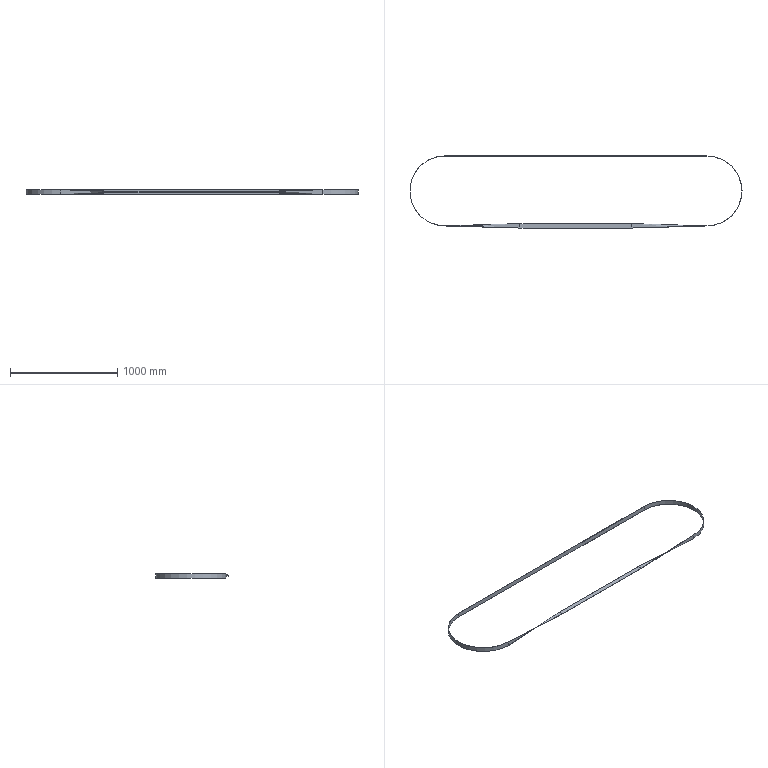Part | SolidWorks | features Blend 2, ICE 1, Sweep 1 | 1 solid | 26 faces | box 3091 x 670.5 x 43 mm | volume 356938 mm3 | plane 12 | spline 8 | cylinder 6 | commonest cylinder face diameters 648.7 x3 651.3 x3
STEP:
#1=CARTESIAN_POINT('',(0.,-325.65,-21.5));
#2=VERTEX_POINT('',#1);
#3=CARTESIAN_POINT('',(325.65,0.,-21.5));
#4=VERTEX_POINT('',#3);
#5=CARTESIAN_POINT('',(0.,0.,-21.5));
#6=DIRECTION('',(0.,0.,1.));
#7=DIRECTION('',(0.,-1.,0.));
#8=AXIS2_PLACEMENT_3D('',#5,#6,#7);
#9=CIRCLE('',#8,325.65);
#10=EDGE_CURVE('',#2,#4,#9,.T.);
#11=ORIENTED_EDGE('',*,*,#10,.T.);
#12=CARTESIAN_POINT('',(325.65,0.,21.5));
#13=VERTEX_POINT('',#12);
#14=CARTESIAN_POINT('',(325.65,0.,0.));
#15=DIRECTION('',(0.,0.,1.));
#16=VECTOR('',#15,1000.);
#17=LINE('',#14,#16);
#18=EDGE_CURVE('',#4,#13,#17,.T.);
#19=ORIENTED_EDGE('',*,*,#18,.T.);
#20=CARTESIAN_POINT('',(0.,-325.65,21.5));
#21=VERTEX_POINT('',#20);
#22=CARTESIAN_POINT('',(0.,0.,21.5));
#23=DIRECTION('',(0.,0.,1.));
#24=DIRECTION('',(0.,-1.,0.));
#25=AXIS2_PLACEMENT_3D('',#22,#23,#24);
#26=CIRCLE('',#25,325.65);
#27=EDGE_CURVE('',#21,#13,#26,.T.);
#28=ORIENTED_EDGE('',*,*,#27,.F.);
#29=CARTESIAN_POINT('',(0.,-325.65,1.363));
#30=VERTEX_POINT('',#29);
#31=CARTESIAN_POINT('',(0.,-325.65,-21.5));
#32=DIRECTION('',(0.,0.,1.));
#33=VECTOR('',#32,1000.);
#34=LINE('',#31,#33);
#35=EDGE_CURVE('',#30,#21,#34,.T.);
#36=ORIENTED_EDGE('',*,*,#35,.F.);
#37=CARTESIAN_POINT('',(0.,-325.65,-21.5));
#38=DIRECTION('',(0.,0.,1.));
#39=VECTOR('',#38,1000.);
#40=LINE('',#37,#39);
#41=EDGE_CURVE('',#2,#30,#40,.T.);
#42=ORIENTED_EDGE('',*,*,#41,.F.);
#43=EDGE_LOOP('',(#11,#19,#28,#36,#42));
#44=FACE_OUTER_BOUND('',#43,.T.);
#45=CARTESIAN_POINT('',(0.,0.,0.));
#46=DIRECTION('',(0.,0.,1.));
#47=DIRECTION('',(1.,0.,0.));
#48=AXIS2_PLACEMENT_3D('',#45,#46,#47);
#49=CYLINDRICAL_SURFACE('',#48,325.65);
#50=ADVANCED_FACE('',(#44),#49,.T.);
#51=CARTESIAN_POINT('',(324.35,0.,-21.5));
#52=VERTEX_POINT('',#51);
#53=CARTESIAN_POINT('',(0.,324.35,-21.5));
#54=VERTEX_POINT('',#53);
#55=CARTESIAN_POINT('',(0.,0.,-21.5));
#56=DIRECTION('',(0.,0.,1.));
#57=DIRECTION('',(0.,-1.,0.));
#58=AXIS2_PLACEMENT_3D('',#55,#56,#57);
#59=CIRCLE('',#58,324.35);
#60=EDGE_CURVE('',#52,#54,#59,.T.);
#61=ORIENTED_EDGE('',*,*,#60,.F.);
#62=CARTESIAN_POINT('',(324.35,0.,21.5));
#63=VERTEX_POINT('',#62);
#64=CARTESIAN_POINT('',(324.35,0.,0.));
#65=DIRECTION('',(0.,0.,1.));
#66=VECTOR('',#65,1000.);
#67=LINE('',#64,#66);
#68=EDGE_CURVE('',#52,#63,#67,.T.);
#69=ORIENTED_EDGE('',*,*,#68,.T.);
#70=CARTESIAN_POINT('',(0.,324.35,21.5));
#71=VERTEX_POINT('',#70);
#72=CARTESIAN_POINT('',(0.,0.,21.5));
#73=DIRECTION('',(0.,0.,1.));
#74=DIRECTION('',(0.,-1.,0.));
#75=AXIS2_PLACEMENT_3D('',#72,#73,#74);
#76=CIRCLE('',#75,324.35);
#77=EDGE_CURVE('',#63,#71,#76,.T.);
#78=ORIENTED_EDGE('',*,*,#77,.T.);
#79=CARTESIAN_POINT('',(0.,324.35,-21.5));
#80=DIRECTION('',(0.,0.,-1.));
#81=VECTOR('',#80,1000.);
#82=LINE('',#79,#81);
#83=EDGE_CURVE('',#71,#54,#82,.T.);
#84=ORIENTED_EDGE('',*,*,#83,.T.);
#85=EDGE_LOOP('',(#61,#69,#78,#84));
#86=FACE_OUTER_BOUND('',#85,.T.);
#87=CARTESIAN_POINT('',(0.,0.,0.));
#88=DIRECTION('',(0.,0.,1.));
#89=DIRECTION('',(1.,0.,0.));
#90=AXIS2_PLACEMENT_3D('',#87,#88,#89);
#91=CYLINDRICAL_SURFACE('',#90,324.35);
#92=ADVANCED_FACE('',(#86),#91,.F.);
#93=CARTESIAN_POINT('',(-2440.,-325.65,-21.5));
#94=VERTEX_POINT('',#93);
#95=CARTESIAN_POINT('',(-2440.,-325.65,21.5));
#96=VERTEX_POINT('',#95);
#97=CARTESIAN_POINT('',(-2440.,-325.65,-21.5));
#98=DIRECTION('',(0.,0.,1.));
#99=VECTOR('',#98,1000.);
#100=LINE('',#97,#99);
#101=EDGE_CURVE('',#94,#96,#100,.T.);
#102=ORIENTED_EDGE('',*,*,#101,.T.);
#103=CARTESIAN_POINT('',(-2440.,325.65,21.5));
#104=VERTEX_POINT('',#103);
#105=CARTESIAN_POINT('',(-2440.,0.,21.5));
#106=DIRECTION('',(0.,0.,1.));
#107=DIRECTION('',(0.,1.,0.));
#108=AXIS2_PLACEMENT_3D('',#105,#106,#107);
#109=CIRCLE('',#108,325.65);
#110=EDGE_CURVE('',#104,#96,#109,.T.);
#111=ORIENTED_EDGE('',*,*,#110,.F.);
#112=CARTESIAN_POINT('',(-2440.,325.65,-21.5));
#113=VERTEX_POINT('',#112);
#114=CARTESIAN_POINT('',(-2440.,325.65,-21.5));
#115=DIRECTION('',(0.,0.,1.));
#116=VECTOR('',#115,1000.);
#117=LINE('',#114,#116);
#118=EDGE_CURVE('',#113,#104,#117,.T.);
#119=ORIENTED_EDGE('',*,*,#118,.F.);
#120=CARTESIAN_POINT('',(-2440.,0.,-21.5));
#121=DIRECTION('',(0.,0.,1.));
#122=DIRECTION('',(0.,1.,0.));
#123=AXIS2_PLACEMENT_3D('',#120,#121,#122);
#124=CIRCLE('',#123,325.65);
#125=EDGE_CURVE('',#113,#94,#124,.T.);
#126=ORIENTED_EDGE('',*,*,#125,.T.);
#127=EDGE_LOOP('',(#102,#111,#119,#126));
#128=FACE_OUTER_BOUND('',#127,.T.);
#129=CARTESIAN_POINT('',(-2440.,0.,0.));
#130=DIRECTION('',(0.,0.,1.));
#131=DIRECTION('',(1.,0.,0.));
#132=AXIS2_PLACEMENT_3D('',#129,#130,#131);
#133=CYLINDRICAL_SURFACE('',#132,325.65);
#134=ADVANCED_FACE('',(#128),#133,.T.);
#135=ORIENTED_EDGE('',*,*,#125,.F.);
#136=CARTESIAN_POINT('',(-2440.,324.35,-21.5));
#137=VERTEX_POINT('',#136);
#138=CARTESIAN_POINT('',(-2440.,325.65,-21.5));
#139=DIRECTION('',(0.,1.,0.));
#140=VECTOR('',#139,1000.);
#141=LINE('',#138,#140);
#142=EDGE_CURVE('',#137,#113,#141,.T.);
#143=ORIENTED_EDGE('',*,*,#142,.F.);
#144=CARTESIAN_POINT('',(-2440.,-324.35,-21.5));
#145=VERTEX_POINT('',#144);
#146=CARTESIAN_POINT('',(-2440.,0.,-21.5));
#147=DIRECTION('',(0.,0.,1.));
#148=DIRECTION('',(0.,1.,0.));
#149=AXIS2_PLACEMENT_3D('',#146,#147,#148);
#150=CIRCLE('',#149,324.35);
#151=EDGE_CURVE('',#137,#145,#150,.T.);
#152=ORIENTED_EDGE('',*,*,#151,.T.);
#153=CARTESIAN_POINT('',(-2440.,-325.65,-21.5));
#154=DIRECTION('',(0.,-1.,0.));
#155=VECTOR('',#154,1000.);
#156=LINE('',#153,#155);
#157=EDGE_CURVE('',#145,#94,#156,.T.);
#158=ORIENTED_EDGE('',*,*,#157,.T.);
#159=EDGE_LOOP('',(#135,#143,#152,#158));
#160=FACE_OUTER_BOUND('',#159,.T.);
#161=CARTESIAN_POINT('',(-2440.,325.65,-21.5));
#162=DIRECTION('',(0.,0.,1.));
#163=DIRECTION('',(1.,0.,0.));
#164=AXIS2_PLACEMENT_3D('',#161,#162,#163);
#165=PLANE('',#164);
#166=ADVANCED_FACE('',(#160),#165,.F.);
#167=ORIENTED_EDGE('',*,*,#151,.F.);
#168=CARTESIAN_POINT('',(-2440.,324.35,21.5));
#169=VERTEX_POINT('',#168);
#170=CARTESIAN_POINT('',(-2440.,324.35,-21.5));
#171=DIRECTION('',(0.,0.,-1.));
#172=VECTOR('',#171,1000.);
#173=LINE('',#170,#172);
#174=EDGE_CURVE('',#169,#137,#173,.T.);
#175=ORIENTED_EDGE('',*,*,#174,.F.);
#176=CARTESIAN_POINT('',(-2440.,-324.35,21.5));
#177=VERTEX_POINT('',#176);
#178=CARTESIAN_POINT('',(-2440.,0.,21.5));
#179=DIRECTION('',(0.,0.,1.));
#180=DIRECTION('',(0.,1.,0.));
#181=AXIS2_PLACEMENT_3D('',#178,#179,#180);
#182=CIRCLE('',#181,324.35);
#183=EDGE_CURVE('',#169,#177,#182,.T.);
#184=ORIENTED_EDGE('',*,*,#183,.T.);
#185=CARTESIAN_POINT('',(-2440.,-324.35,-21.5));
#186=DIRECTION('',(0.,0.,-1.));
#187=VECTOR('',#186,1000.);
#188=LINE('',#185,#187);
#189=EDGE_CURVE('',#177,#145,#188,.T.);
#190=ORIENTED_EDGE('',*,*,#189,.T.);
#191=EDGE_LOOP('',(#167,#175,#184,#190));
#192=FACE_OUTER_BOUND('',#191,.T.);
#193=CARTESIAN_POINT('',(-2440.,0.,0.));
#194=DIRECTION('',(0.,0.,1.));
#195=DIRECTION('',(1.,0.,0.));
#196=AXIS2_PLACEMENT_3D('',#193,#194,#195);
#197=CYLINDRICAL_SURFACE('',#196,324.35);
#198=ADVANCED_FACE('',(#192),#197,.F.);
#199=ORIENTED_EDGE('',*,*,#183,.F.);
#200=CARTESIAN_POINT('',(-2440.,325.65,21.5));
#201=DIRECTION('',(0.,-1.,0.));
#202=VECTOR('',#201,1000.);
#203=LINE('',#200,#202);
#204=EDGE_CURVE('',#104,#169,#203,.T.);
#205=ORIENTED_EDGE('',*,*,#204,.F.);
#206=ORIENTED_EDGE('',*,*,#110,.T.);
#207=CARTESIAN_POINT('',(-2440.,-325.65,21.5));
#208=DIRECTION('',(0.,1.,0.));
#209=VECTOR('',#208,1000.);
#210=LINE('',#207,#209);
#211=EDGE_CURVE('',#96,#177,#210,.T.);
#212=ORIENTED_EDGE('',*,*,#211,.T.);
#213=EDGE_LOOP('',(#199,#205,#206,#212));
#214=FACE_OUTER_BOUND('',#213,.T.);
#215=CARTESIAN_POINT('',(-2440.,325.65,21.5));
#216=DIRECTION('',(0.,0.,-1.));
#217=DIRECTION('',(-1.,0.,0.));
#218=AXIS2_PLACEMENT_3D('',#215,#216,#217);
#219=PLANE('',#218);
#220=ADVANCED_FACE('',(#214),#219,.F.);
#221=ORIENTED_EDGE('',*,*,#118,.T.);
#222=CARTESIAN_POINT('',(0.,325.65,21.5));
#223=VERTEX_POINT('',#222);
#224=CARTESIAN_POINT('',(0.,325.65,21.5));
#225=DIRECTION('',(-1.,0.,0.));
#226=VECTOR('',#225,1000.);
#227=LINE('',#224,#226);
#228=EDGE_CURVE('',#223,#104,#227,.T.);
#229=ORIENTED_EDGE('',*,*,#228,.F.);
#230=CARTESIAN_POINT('',(0.,325.65,-21.5));
#231=VERTEX_POINT('',#230);
#232=CARTESIAN_POINT('',(0.,325.65,-21.5));
#233=DIRECTION('',(0.,0.,1.));
#234=VECTOR('',#233,1000.);
#235=LINE('',#232,#234);
#236=EDGE_CURVE('',#231,#223,#235,.T.);
#237=ORIENTED_EDGE('',*,*,#236,.F.);
#238=CARTESIAN_POINT('',(0.,325.65,-21.5));
#239=DIRECTION('',(-1.,0.,0.));
#240=VECTOR('',#239,1000.);
#241=LINE('',#238,#240);
#242=EDGE_CURVE('',#231,#113,#241,.T.);
#243=ORIENTED_EDGE('',*,*,#242,.T.);
#244=EDGE_LOOP('',(#221,#229,#237,#243));
#245=FACE_OUTER_BOUND('',#244,.T.);
#246=CARTESIAN_POINT('',(0.,325.65,-21.5));
#247=DIRECTION('',(0.,-1.,0.));
#248=DIRECTION('',(1.,0.,0.));
#249=AXIS2_PLACEMENT_3D('',#246,#247,#248);
#250=PLANE('',#249);
#251=ADVANCED_FACE('',(#245),#250,.F.);
#252=ORIENTED_EDGE('',*,*,#242,.F.);
#253=CARTESIAN_POINT('',(0.,325.65,-21.5));
#254=DIRECTION('',(0.,1.,0.));
#255=VECTOR('',#254,1000.);
#256=LINE('',#253,#255);
#257=EDGE_CURVE('',#54,#231,#256,.T.);
#258=ORIENTED_EDGE('',*,*,#257,.F.);
#259=CARTESIAN_POINT('',(0.,324.35,-21.5));
#260=DIRECTION('',(-1.,0.,0.));
#261=VECTOR('',#260,1000.);
#262=LINE('',#259,#261);
#263=EDGE_CURVE('',#54,#137,#262,.T.);
#264=ORIENTED_EDGE('',*,*,#263,.T.);
#265=ORIENTED_EDGE('',*,*,#142,.T.);
#266=EDGE_LOOP('',(#252,#258,#264,#265));
#267=FACE_OUTER_BOUND('',#266,.T.);
#268=CARTESIAN_POINT('',(0.,325.65,-21.5));
#269=DIRECTION('',(0.,0.,1.));
#270=DIRECTION('',(1.,0.,0.));
#271=AXIS2_PLACEMENT_3D('',#268,#269,#270);
#272=PLANE('',#271);
#273=ADVANCED_FACE('',(#267),#272,.F.);
#274=ORIENTED_EDGE('',*,*,#263,.F.);
#275=ORIENTED_EDGE('',*,*,#83,.F.);
#276=CARTESIAN_POINT('',(0.,324.35,21.5));
#277=DIRECTION('',(-1.,0.,0.));
#278=VECTOR('',#277,1000.);
#279=LINE('',#276,#278);
#280=EDGE_CURVE('',#71,#169,#279,.T.);
#281=ORIENTED_EDGE('',*,*,#280,.T.);
#282=ORIENTED_EDGE('',*,*,#174,.T.);
#283=EDGE_LOOP('',(#274,#275,#281,#282));
#284=FACE_OUTER_BOUND('',#283,.T.);
#285=CARTESIAN_POINT('',(0.,324.35,-21.5));
#286=DIRECTION('',(0.,1.,0.));
#287=DIRECTION('',(0.,0.,1.));
#288=AXIS2_PLACEMENT_3D('',#285,#286,#287);
#289=PLANE('',#288);
#290=ADVANCED_FACE('',(#284),#289,.F.);
#291=ORIENTED_EDGE('',*,*,#280,.F.);
#292=CARTESIAN_POINT('',(0.,325.65,21.5));
#293=DIRECTION('',(0.,-1.,0.));
#294=VECTOR('',#293,1000.);
#295=LINE('',#292,#294);
#296=EDGE_CURVE('',#223,#71,#295,.T.);
#297=ORIENTED_EDGE('',*,*,#296,.F.);
#298=ORIENTED_EDGE('',*,*,#228,.T.);
#299=ORIENTED_EDGE('',*,*,#204,.T.);
#300=EDGE_LOOP('',(#291,#297,#298,#299));
#301=FACE_OUTER_BOUND('',#300,.T.);
#302=CARTESIAN_POINT('',(0.,325.65,21.5));
#303=DIRECTION('',(0.,0.,-1.));
#304=DIRECTION('',(-1.,0.,0.));
#305=AXIS2_PLACEMENT_3D('',#302,#303,#304);
#306=PLANE('',#305);
#307=ADVANCED_FACE('',(#301),#306,.F.);
#308=ORIENTED_EDGE('',*,*,#18,.F.);
#309=CARTESIAN_POINT('',(0.,0.,-21.5));
#310=DIRECTION('',(0.,0.,1.));
#311=DIRECTION('',(0.,-1.,0.));
#312=AXIS2_PLACEMENT_3D('',#309,#310,#311);
#313=CIRCLE('',#312,325.65);
#314=EDGE_CURVE('',#4,#231,#313,.T.);
#315=ORIENTED_EDGE('',*,*,#314,.T.);
#316=ORIENTED_EDGE('',*,*,#236,.T.);
#317=CARTESIAN_POINT('',(0.,0.,21.5));
#318=DIRECTION('',(0.,0.,1.));
#319=DIRECTION('',(0.,-1.,0.));
#320=AXIS2_PLACEMENT_3D('',#317,#318,#319);
#321=CIRCLE('',#320,325.65);
#322=EDGE_CURVE('',#13,#223,#321,.T.);
#323=ORIENTED_EDGE('',*,*,#322,.F.);
#324=EDGE_LOOP('',(#308,#315,#316,#323));
#325=FACE_OUTER_BOUND('',#324,.T.);
#326=CARTESIAN_POINT('',(0.,0.,0.));
#327=DIRECTION('',(0.,0.,1.));
#328=DIRECTION('',(1.,0.,0.));
#329=AXIS2_PLACEMENT_3D('',#326,#327,#328);
#330=CYLINDRICAL_SURFACE('',#329,325.65);
#331=ADVANCED_FACE('',(#325),#330,.T.);
#332=ORIENTED_EDGE('',*,*,#10,.F.);
#333=CARTESIAN_POINT('',(0.,-324.35,-21.5));
#334=VERTEX_POINT('',#333);
#335=CARTESIAN_POINT('',(0.,-325.65,-21.5));
#336=DIRECTION('',(0.,-1.,0.));
#337=VECTOR('',#336,1000.);
#338=LINE('',#335,#337);
#339=EDGE_CURVE('',#334,#2,#338,.T.);
#340=ORIENTED_EDGE('',*,*,#339,.F.);
#341=CARTESIAN_POINT('',(0.,0.,-21.5));
#342=DIRECTION('',(0.,0.,1.));
#343=DIRECTION('',(0.,-1.,0.));
#344=AXIS2_PLACEMENT_3D('',#341,#342,#343);
#345=CIRCLE('',#344,324.35);
#346=EDGE_CURVE('',#334,#52,#345,.T.);
#347=ORIENTED_EDGE('',*,*,#346,.T.);
#348=ORIENTED_EDGE('',*,*,#60,.T.);
#349=ORIENTED_EDGE('',*,*,#257,.T.);
#350=ORIENTED_EDGE('',*,*,#314,.F.);
#351=EDGE_LOOP('',(#332,#340,#347,#348,#349,#350));
#352=FACE_OUTER_BOUND('',#351,.T.);
#353=CARTESIAN_POINT('',(0.,-325.65,-21.5));
#354=DIRECTION('',(0.,0.,1.));
#355=DIRECTION('',(1.,0.,0.));
#356=AXIS2_PLACEMENT_3D('',#353,#354,#355);
#357=PLANE('',#356);
#358=ADVANCED_FACE('',(#352),#357,.F.);
#359=ORIENTED_EDGE('',*,*,#68,.F.);
#360=ORIENTED_EDGE('',*,*,#346,.F.);
#361=CARTESIAN_POINT('',(0.,-324.35,0.));
#362=VERTEX_POINT('',#361);
#363=CARTESIAN_POINT('',(0.,-324.35,-21.5));
#364=DIRECTION('',(0.,0.,-1.));
#365=VECTOR('',#364,1000.);
#366=LINE('',#363,#365);
#367=EDGE_CURVE('',#362,#334,#366,.T.);
#368=ORIENTED_EDGE('',*,*,#367,.F.);
#369=CARTESIAN_POINT('',(0.,-324.35,21.5));
#370=VERTEX_POINT('',#369);
#371=CARTESIAN_POINT('',(0.,-324.35,-21.5));
#372=DIRECTION('',(0.,0.,-1.));
#373=VECTOR('',#372,1000.);
#374=LINE('',#371,#373);
#375=EDGE_CURVE('',#370,#362,#374,.T.);
#376=ORIENTED_EDGE('',*,*,#375,.F.);
#377=CARTESIAN_POINT('',(0.,0.,21.5));
#378=DIRECTION('',(0.,0.,1.));
#379=DIRECTION('',(0.,-1.,0.));
#380=AXIS2_PLACEMENT_3D('',#377,#378,#379);
#381=CIRCLE('',#380,324.35);
#382=EDGE_CURVE('',#370,#63,#381,.T.);
#383=ORIENTED_EDGE('',*,*,#382,.T.);
#384=EDGE_LOOP('',(#359,#360,#368,#376,#383));
#385=FACE_OUTER_BOUND('',#384,.T.);
#386=CARTESIAN_POINT('',(0.,0.,0.));
#387=DIRECTION('',(0.,0.,1.));
#388=DIRECTION('',(1.,0.,0.));
#389=AXIS2_PLACEMENT_3D('',#386,#387,#388);
#390=CYLINDRICAL_SURFACE('',#389,324.35);
#391=ADVANCED_FACE('',(#385),#390,.F.);
#392=ORIENTED_EDGE('',*,*,#382,.F.);
#393=CARTESIAN_POINT('',(0.,-325.65,21.5));
#394=DIRECTION('',(0.,1.,0.));
#395=VECTOR('',#394,1000.);
#396=LINE('',#393,#395);
#397=EDGE_CURVE('',#21,#370,#396,.T.);
#398=ORIENTED_EDGE('',*,*,#397,.F.);
#399=ORIENTED_EDGE('',*,*,#27,.T.);
#400=ORIENTED_EDGE('',*,*,#322,.T.);
#401=ORIENTED_EDGE('',*,*,#296,.T.);
#402=ORIENTED_EDGE('',*,*,#77,.F.);
#403=EDGE_LOOP('',(#392,#398,#399,#400,#401,#402));
#404=FACE_OUTER_BOUND('',#403,.T.);
#405=CARTESIAN_POINT('',(0.,-325.65,21.5));
#406=DIRECTION('',(0.,0.,-1.));
#407=DIRECTION('',(-1.,0.,0.));
#408=AXIS2_PLACEMENT_3D('',#405,#406,#407);
#409=PLANE('',#408);
#410=ADVANCED_FACE('',(#404),#409,.F.);
#411=CARTESIAN_POINT('',(-700.,-303.85,-0.65));
#412=VERTEX_POINT('',#411);
#413=CARTESIAN_POINT('',(-700.,-344.85,-0.65));
#414=VERTEX_POINT('',#413);
#415=CARTESIAN_POINT('',(-700.,-344.85,-0.65));
#416=DIRECTION('',(0.,-1.,0.));
#417=VECTOR('',#416,1000.);
#418=LINE('',#415,#417);
#419=EDGE_CURVE('',#412,#414,#418,.T.);
#420=ORIENTED_EDGE('',*,*,#419,.F.);
#421=CARTESIAN_POINT('',(-350.,-314.75,-11.075));
#422=DIRECTION('',(0.9991,-0.03111,-0.02976));
#423=VECTOR('',#422,1000.);
#424=LINE('',#421,#423);
#425=EDGE_CURVE('',#412,#2,#424,.T.);
#426=ORIENTED_EDGE('',*,*,#425,.T.);
#427=ORIENTED_EDGE('',*,*,#41,.T.);
#428=ORIENTED_EDGE('',*,*,#35,.T.);
#429=CARTESIAN_POINT('',(-350.,-335.25,10.425));
#430=DIRECTION('',(-0.9991,-0.0274,-0.03162));
#431=VECTOR('',#430,1000.);
#432=LINE('',#429,#431);
#433=EDGE_CURVE('',#21,#414,#432,.T.);
#434=ORIENTED_EDGE('',*,*,#433,.T.);
#435=EDGE_LOOP('',(#420,#426,#427,#428,#434));
#436=FACE_OUTER_BOUND('',#435,.T.);
#437=CARTESIAN_POINT('',(-700.,-344.85,-0.65));
#438=CARTESIAN_POINT('',(0.,-325.65,21.5));
#439=CARTESIAN_POINT('',(-700.,-338.017,-0.65));
#440=CARTESIAN_POINT('',(0.,-325.65,14.333));
#441=CARTESIAN_POINT('',(-700.,-331.183,-0.65));
#442=CARTESIAN_POINT('',(0.,-325.65,7.167));
#443=CARTESIAN_POINT('',(-700.,-317.517,-0.65));
#444=CARTESIAN_POINT('',(0.,-325.65,-7.167));
#445=CARTESIAN_POINT('',(-700.,-310.683,-0.65));
#446=CARTESIAN_POINT('',(0.,-325.65,-14.333));
#447=CARTESIAN_POINT('',(-700.,-303.85,-0.65));
#448=CARTESIAN_POINT('',(0.,-325.65,-21.5));
#449=B_SPLINE_SURFACE_WITH_KNOTS('',3,1,((#437,#438),(#439,#440),(#441,#442),(#443,#444),(#445,#446),(#447,#448)),.UNSPECIFIED.,.F.,.F.,.F.,(4,2,4),(2,2),(0.,0.5,1.),(0.,1.),.UNSPECIFIED.);
#450=ADVANCED_FACE('',(#436),#449,.T.);
#451=CARTESIAN_POINT('',(-700.,-303.85,0.65));
#452=VERTEX_POINT('',#451);
#453=CARTESIAN_POINT('',(-700.,-303.85,-0.65));
#454=DIRECTION('',(0.,0.,-1.));
#455=VECTOR('',#454,1000.);
#456=LINE('',#453,#455);
#457=EDGE_CURVE('',#452,#412,#456,.T.);
#458=ORIENTED_EDGE('',*,*,#457,.F.);
#459=CARTESIAN_POINT('',(-350.,-314.1,-10.425));
#460=DIRECTION('',(0.9991,-0.02926,-0.03161));
#461=VECTOR('',#460,1000.);
#462=LINE('',#459,#461);
#463=EDGE_CURVE('',#452,#334,#462,.T.);
#464=ORIENTED_EDGE('',*,*,#463,.T.);
#465=ORIENTED_EDGE('',*,*,#339,.T.);
#466=ORIENTED_EDGE('',*,*,#425,.F.);
#467=EDGE_LOOP('',(#458,#464,#465,#466));
#468=FACE_OUTER_BOUND('',#467,.T.);
#469=CARTESIAN_POINT('',(-700.,-303.85,-0.65));
#470=CARTESIAN_POINT('',(0.,-325.65,-21.5));
#471=CARTESIAN_POINT('',(-700.,-303.85,-0.4333));
#472=CARTESIAN_POINT('',(0.,-325.433,-21.5));
#473=CARTESIAN_POINT('',(-700.,-303.85,-0.2167));
#474=CARTESIAN_POINT('',(0.,-325.217,-21.5));
#475=CARTESIAN_POINT('',(-700.,-303.85,0.2167));
#476=CARTESIAN_POINT('',(0.,-324.783,-21.5));
#477=CARTESIAN_POINT('',(-700.,-303.85,0.4333));
#478=CARTESIAN_POINT('',(0.,-324.567,-21.5));
#479=CARTESIAN_POINT('',(-700.,-303.85,0.65));
#480=CARTESIAN_POINT('',(0.,-324.35,-21.5));
#481=B_SPLINE_SURFACE_WITH_KNOTS('',3,1,((#469,#470),(#471,#472),(#473,#474),(#475,#476),(#477,#478),(#479,#480)),.UNSPECIFIED.,.F.,.F.,.F.,(4,2,4),(2,2),(0.,0.5,1.),(0.,1.),.UNSPECIFIED.);
#482=ADVANCED_FACE('',(#468),#481,.T.);
#483=CARTESIAN_POINT('',(-700.,-344.85,0.65));
#484=VERTEX_POINT('',#483);
#485=CARTESIAN_POINT('',(-700.,-344.85,-0.65));
#486=DIRECTION('',(0.,0.,1.));
#487=VECTOR('',#486,1000.);
#488=LINE('',#485,#487);
#489=EDGE_CURVE('',#414,#484,#488,.T.);
#490=ORIENTED_EDGE('',*,*,#489,.F.);
#491=ORIENTED_EDGE('',*,*,#433,.F.);
#492=ORIENTED_EDGE('',*,*,#397,.T.);
#493=CARTESIAN_POINT('',(-350.,-334.6,11.075));
#494=DIRECTION('',(0.9991,0.02926,0.02976));
#495=VECTOR('',#494,1000.);
#496=LINE('',#493,#495);
#497=EDGE_CURVE('',#484,#370,#496,.T.);
#498=ORIENTED_EDGE('',*,*,#497,.F.);
#499=EDGE_LOOP('',(#490,#491,#492,#498));
#500=FACE_OUTER_BOUND('',#499,.T.);
#501=CARTESIAN_POINT('',(-700.,-344.85,0.65));
#502=CARTESIAN_POINT('',(0.,-324.35,21.5));
#503=CARTESIAN_POINT('',(-700.,-344.85,0.4333));
#504=CARTESIAN_POINT('',(0.,-324.567,21.5));
#505=CARTESIAN_POINT('',(-700.,-344.85,0.2167));
#506=CARTESIAN_POINT('',(0.,-324.783,21.5));
#507=CARTESIAN_POINT('',(-700.,-344.85,-0.2167));
#508=CARTESIAN_POINT('',(0.,-325.217,21.5));
#509=CARTESIAN_POINT('',(-700.,-344.85,-0.4333));
#510=CARTESIAN_POINT('',(0.,-325.433,21.5));
#511=CARTESIAN_POINT('',(-700.,-344.85,-0.65));
#512=CARTESIAN_POINT('',(0.,-325.65,21.5));
#513=B_SPLINE_SURFACE_WITH_KNOTS('',3,1,((#501,#502),(#503,#504),(#505,#506),(#507,#508),(#509,#510),(#511,#512)),.UNSPECIFIED.,.F.,.F.,.F.,(4,2,4),(2,2),(0.,0.5,1.),(0.,1.),.UNSPECIFIED.);
#514=ADVANCED_FACE('',(#500),#513,.T.);
#515=CARTESIAN_POINT('',(-700.,-344.85,0.65));
#516=DIRECTION('',(0.,1.,0.));
#517=VECTOR('',#516,1000.);
#518=LINE('',#515,#517);
#519=EDGE_CURVE('',#484,#452,#518,.T.);
#520=ORIENTED_EDGE('',*,*,#519,.F.);
#521=ORIENTED_EDGE('',*,*,#497,.T.);
#522=ORIENTED_EDGE('',*,*,#375,.T.);
#523=ORIENTED_EDGE('',*,*,#367,.T.);
#524=ORIENTED_EDGE('',*,*,#463,.F.);
#525=EDGE_LOOP('',(#520,#521,#522,#523,#524));
#526=FACE_OUTER_BOUND('',#525,.T.);
#527=CARTESIAN_POINT('',(-700.,-303.85,0.65));
#528=CARTESIAN_POINT('',(0.,-324.35,-21.5));
#529=CARTESIAN_POINT('',(-700.,-310.683,0.65));
#530=CARTESIAN_POINT('',(0.,-324.35,-14.333));
#531=CARTESIAN_POINT('',(-700.,-317.517,0.65));
#532=CARTESIAN_POINT('',(0.,-324.35,-7.167));
#533=CARTESIAN_POINT('',(-700.,-331.183,0.65));
#534=CARTESIAN_POINT('',(0.,-324.35,7.167));
#535=CARTESIAN_POINT('',(-700.,-338.017,0.65));
#536=CARTESIAN_POINT('',(0.,-324.35,14.333));
#537=CARTESIAN_POINT('',(-700.,-344.85,0.65));
#538=CARTESIAN_POINT('',(0.,-324.35,21.5));
#539=B_SPLINE_SURFACE_WITH_KNOTS('',3,1,((#527,#528),(#529,#530),(#531,#532),(#533,#534),(#535,#536),(#537,#538)),.UNSPECIFIED.,.F.,.F.,.F.,(4,2,4),(2,2),(0.,0.5,1.),(0.,1.),.UNSPECIFIED.);
#540=ADVANCED_FACE('',(#526),#539,.T.);
#541=CARTESIAN_POINT('',(-1740.,-344.85,-0.65));
#542=VERTEX_POINT('',#541);
#543=CARTESIAN_POINT('',(-1781.021,-344.85,-0.65));
#544=DIRECTION('',(1.,0.,0.));
#545=VECTOR('',#544,1000.);
#546=LINE('',#543,#545);
#547=EDGE_CURVE('',#542,#414,#546,.T.);
#548=ORIENTED_EDGE('',*,*,#547,.F.);
#549=CARTESIAN_POINT('',(-1740.,-303.85,-0.65));
#550=VERTEX_POINT('',#549);
#551=CARTESIAN_POINT('',(-1740.,-344.85,-0.65));
#552=DIRECTION('',(0.,1.,0.));
#553=VECTOR('',#552,1000.);
#554=LINE('',#551,#553);
#555=EDGE_CURVE('',#542,#550,#554,.T.);
#556=ORIENTED_EDGE('',*,*,#555,.T.);
#557=CARTESIAN_POINT('',(-1781.021,-303.85,-0.65));
#558=DIRECTION('',(1.,0.,0.));
#559=VECTOR('',#558,1000.);
#560=LINE('',#557,#559);
#561=EDGE_CURVE('',#550,#412,#560,.T.);
#562=ORIENTED_EDGE('',*,*,#561,.T.);
#563=ORIENTED_EDGE('',*,*,#419,.T.);
#564=EDGE_LOOP('',(#548,#556,#562,#563));
#565=FACE_OUTER_BOUND('',#564,.T.);
#566=CARTESIAN_POINT('',(-1781.021,-344.85,-0.65));
#567=DIRECTION('',(0.,0.,1.));
#568=DIRECTION('',(0.,-1.,0.));
#569=AXIS2_PLACEMENT_3D('',#566,#567,#568);
#570=PLANE('',#569);
#571=ADVANCED_FACE('',(#565),#570,.F.);
#572=ORIENTED_EDGE('',*,*,#561,.F.);
#573=CARTESIAN_POINT('',(-1740.,-303.85,0.65));
#574=VERTEX_POINT('',#573);
#575=CARTESIAN_POINT('',(-1740.,-303.85,-0.65));
#576=DIRECTION('',(0.,0.,1.));
#577=VECTOR('',#576,1000.);
#578=LINE('',#575,#577);
#579=EDGE_CURVE('',#550,#574,#578,.T.);
#580=ORIENTED_EDGE('',*,*,#579,.T.);
#581=CARTESIAN_POINT('',(-1781.021,-303.85,0.65));
#582=DIRECTION('',(1.,0.,0.));
#583=VECTOR('',#582,1000.);
#584=LINE('',#581,#583);
#585=EDGE_CURVE('',#574,#452,#584,.T.);
#586=ORIENTED_EDGE('',*,*,#585,.T.);
#587=ORIENTED_EDGE('',*,*,#457,.T.);
#588=EDGE_LOOP('',(#572,#580,#586,#587));
#589=FACE_OUTER_BOUND('',#588,.T.);
#590=CARTESIAN_POINT('',(-1781.021,-303.85,-0.65));
#591=DIRECTION('',(0.,-1.,0.));
#592=DIRECTION('',(0.,0.,-1.));
#593=AXIS2_PLACEMENT_3D('',#590,#591,#592);
#594=PLANE('',#593);
#595=ADVANCED_FACE('',(#589),#594,.F.);
#596=ORIENTED_EDGE('',*,*,#585,.F.);
#597=CARTESIAN_POINT('',(-1740.,-344.85,0.65));
#598=VERTEX_POINT('',#597);
#599=CARTESIAN_POINT('',(-1740.,-344.85,0.65));
#600=DIRECTION('',(0.,-1.,0.));
#601=VECTOR('',#600,1000.);
#602=LINE('',#599,#601);
#603=EDGE_CURVE('',#574,#598,#602,.T.);
#604=ORIENTED_EDGE('',*,*,#603,.T.);
#605=CARTESIAN_POINT('',(-1781.021,-344.85,0.65));
#606=DIRECTION('',(1.,0.,0.));
#607=VECTOR('',#606,1000.);
#608=LINE('',#605,#607);
#609=EDGE_CURVE('',#598,#484,#608,.T.);
#610=ORIENTED_EDGE('',*,*,#609,.T.);
#611=ORIENTED_EDGE('',*,*,#519,.T.);
#612=EDGE_LOOP('',(#596,#604,#610,#611));
#613=FACE_OUTER_BOUND('',#612,.T.);
#614=CARTESIAN_POINT('',(-1781.021,-344.85,0.65));
#615=DIRECTION('',(0.,0.,-1.));
#616=DIRECTION('',(0.,1.,0.));
#617=AXIS2_PLACEMENT_3D('',#614,#615,#616);
#618=PLANE('',#617);
#619=ADVANCED_FACE('',(#613),#618,.F.);
#620=ORIENTED_EDGE('',*,*,#609,.F.);
#621=CARTESIAN_POINT('',(-1740.,-344.85,-0.65));
#622=DIRECTION('',(0.,0.,-1.));
#623=VECTOR('',#622,1000.);
#624=LINE('',#621,#623);
#625=EDGE_CURVE('',#598,#542,#624,.T.);
#626=ORIENTED_EDGE('',*,*,#625,.T.);
#627=ORIENTED_EDGE('',*,*,#547,.T.);
#628=ORIENTED_EDGE('',*,*,#489,.T.);
#629=EDGE_LOOP('',(#620,#626,#627,#628));
#630=FACE_OUTER_BOUND('',#629,.T.);
#631=CARTESIAN_POINT('',(-1781.021,-344.85,-0.65));
#632=DIRECTION('',(0.,1.,0.));
#633=DIRECTION('',(0.,0.,1.));
#634=AXIS2_PLACEMENT_3D('',#631,#632,#633);
#635=PLANE('',#634);
#636=ADVANCED_FACE('',(#630),#635,.F.);
#637=ORIENTED_EDGE('',*,*,#211,.F.);
#638=CARTESIAN_POINT('',(-2090.,-335.25,10.425));
#639=DIRECTION('',(0.9991,-0.0274,-0.03162));
#640=VECTOR('',#639,1000.);
#641=LINE('',#638,#640);
#642=EDGE_CURVE('',#96,#542,#641,.T.);
#643=ORIENTED_EDGE('',*,*,#642,.T.);
#644=ORIENTED_EDGE('',*,*,#625,.F.);
#645=CARTESIAN_POINT('',(-2090.,-334.6,11.075));
#646=DIRECTION('',(-0.9991,0.02926,0.02976));
#647=VECTOR('',#646,1000.);
#648=LINE('',#645,#647);
#649=EDGE_CURVE('',#598,#177,#648,.T.);
#650=ORIENTED_EDGE('',*,*,#649,.T.);
#651=EDGE_LOOP('',(#637,#643,#644,#650));
#652=FACE_OUTER_BOUND('',#651,.T.);
#653=CARTESIAN_POINT('',(-2440.,-324.35,21.5));
#654=CARTESIAN_POINT('',(-1740.,-344.85,0.65));
#655=CARTESIAN_POINT('',(-2440.,-324.567,21.5));
#656=CARTESIAN_POINT('',(-1740.,-344.85,0.4333));
#657=CARTESIAN_POINT('',(-2440.,-324.783,21.5));
#658=CARTESIAN_POINT('',(-1740.,-344.85,0.2167));
#659=CARTESIAN_POINT('',(-2440.,-325.217,21.5));
#660=CARTESIAN_POINT('',(-1740.,-344.85,-0.2167));
#661=CARTESIAN_POINT('',(-2440.,-325.433,21.5));
#662=CARTESIAN_POINT('',(-1740.,-344.85,-0.4333));
#663=CARTESIAN_POINT('',(-2440.,-325.65,21.5));
#664=CARTESIAN_POINT('',(-1740.,-344.85,-0.65));
#665=B_SPLINE_SURFACE_WITH_KNOTS('',3,1,((#653,#654),(#655,#656),(#657,#658),(#659,#660),(#661,#662),(#663,#664)),.UNSPECIFIED.,.F.,.F.,.F.,(4,2,4),(2,2),(0.,0.5,1.),(0.,1.),.UNSPECIFIED.);
#666=ADVANCED_FACE('',(#652),#665,.T.);
#667=ORIENTED_EDGE('',*,*,#101,.F.);
#668=CARTESIAN_POINT('',(-2090.,-314.75,-11.075));
#669=DIRECTION('',(0.9991,0.03111,0.02976));
#670=VECTOR('',#669,1000.);
#671=LINE('',#668,#670);
#672=EDGE_CURVE('',#94,#550,#671,.T.);
#673=ORIENTED_EDGE('',*,*,#672,.T.);
#674=ORIENTED_EDGE('',*,*,#555,.F.);
#675=ORIENTED_EDGE('',*,*,#642,.F.);
#676=EDGE_LOOP('',(#667,#673,#674,#675));
#677=FACE_OUTER_BOUND('',#676,.T.);
#678=CARTESIAN_POINT('',(-2440.,-325.65,21.5));
#679=CARTESIAN_POINT('',(-1740.,-344.85,-0.65));
#680=CARTESIAN_POINT('',(-2440.,-325.65,14.333));
#681=CARTESIAN_POINT('',(-1740.,-338.017,-0.65));
#682=CARTESIAN_POINT('',(-2440.,-325.65,7.167));
#683=CARTESIAN_POINT('',(-1740.,-331.183,-0.65));
#684=CARTESIAN_POINT('',(-2440.,-325.65,-7.167));
#685=CARTESIAN_POINT('',(-1740.,-317.517,-0.65));
#686=CARTESIAN_POINT('',(-2440.,-325.65,-14.333));
#687=CARTESIAN_POINT('',(-1740.,-310.683,-0.65));
#688=CARTESIAN_POINT('',(-2440.,-325.65,-21.5));
#689=CARTESIAN_POINT('',(-1740.,-303.85,-0.65));
#690=B_SPLINE_SURFACE_WITH_KNOTS('',3,1,((#678,#679),(#680,#681),(#682,#683),(#684,#685),(#686,#687),(#688,#689)),.UNSPECIFIED.,.F.,.F.,.F.,(4,2,4),(2,2),(0.,0.5,1.),(0.,1.),.UNSPECIFIED.);
#691=ADVANCED_FACE('',(#677),#690,.T.);
#692=ORIENTED_EDGE('',*,*,#189,.F.);
#693=ORIENTED_EDGE('',*,*,#649,.F.);
#694=ORIENTED_EDGE('',*,*,#603,.F.);
#695=CARTESIAN_POINT('',(-2090.,-314.1,-10.425));
#696=DIRECTION('',(0.9991,0.02926,0.03161));
#697=VECTOR('',#696,1000.);
#698=LINE('',#695,#697);
#699=EDGE_CURVE('',#145,#574,#698,.T.);
#700=ORIENTED_EDGE('',*,*,#699,.F.);
#701=EDGE_LOOP('',(#692,#693,#694,#700));
#702=FACE_OUTER_BOUND('',#701,.T.);
#703=CARTESIAN_POINT('',(-2440.,-324.35,-21.5));
#704=CARTESIAN_POINT('',(-1740.,-303.85,0.65));
#705=CARTESIAN_POINT('',(-2440.,-324.35,-14.333));
#706=CARTESIAN_POINT('',(-1740.,-310.683,0.65));
#707=CARTESIAN_POINT('',(-2440.,-324.35,-7.167));
#708=CARTESIAN_POINT('',(-1740.,-317.517,0.65));
#709=CARTESIAN_POINT('',(-2440.,-324.35,7.167));
#710=CARTESIAN_POINT('',(-1740.,-331.183,0.65));
#711=CARTESIAN_POINT('',(-2440.,-324.35,14.333));
#712=CARTESIAN_POINT('',(-1740.,-338.017,0.65));
#713=CARTESIAN_POINT('',(-2440.,-324.35,21.5));
#714=CARTESIAN_POINT('',(-1740.,-344.85,0.65));
#715=B_SPLINE_SURFACE_WITH_KNOTS('',3,1,((#703,#704),(#705,#706),(#707,#708),(#709,#710),(#711,#712),(#713,#714)),.UNSPECIFIED.,.F.,.F.,.F.,(4,2,4),(2,2),(0.,0.5,1.),(0.,1.),.UNSPECIFIED.);
#716=ADVANCED_FACE('',(#702),#715,.T.);
#717=ORIENTED_EDGE('',*,*,#157,.F.);
#718=ORIENTED_EDGE('',*,*,#699,.T.);
#719=ORIENTED_EDGE('',*,*,#579,.F.);
#720=ORIENTED_EDGE('',*,*,#672,.F.);
#721=EDGE_LOOP('',(#717,#718,#719,#720));
#722=FACE_OUTER_BOUND('',#721,.T.);
#723=CARTESIAN_POINT('',(-2440.,-325.65,-21.5));
#724=CARTESIAN_POINT('',(-1740.,-303.85,-0.65));
#725=CARTESIAN_POINT('',(-2440.,-325.433,-21.5));
#726=CARTESIAN_POINT('',(-1740.,-303.85,-0.4333));
#727=CARTESIAN_POINT('',(-2440.,-325.217,-21.5));
#728=CARTESIAN_POINT('',(-1740.,-303.85,-0.2167));
#729=CARTESIAN_POINT('',(-2440.,-324.783,-21.5));
#730=CARTESIAN_POINT('',(-1740.,-303.85,0.2167));
#731=CARTESIAN_POINT('',(-2440.,-324.567,-21.5));
#732=CARTESIAN_POINT('',(-1740.,-303.85,0.4333));
#733=CARTESIAN_POINT('',(-2440.,-324.35,-21.5));
#734=CARTESIAN_POINT('',(-1740.,-303.85,0.65));
#735=B_SPLINE_SURFACE_WITH_KNOTS('',3,1,((#723,#724),(#725,#726),(#727,#728),(#729,#730),(#731,#732),(#733,#734)),.UNSPECIFIED.,.F.,.F.,.F.,(4,2,4),(2,2),(0.,0.5,1.),(0.,1.),.UNSPECIFIED.);
#736=ADVANCED_FACE('',(#722),#735,.T.);
#737=CLOSED_SHELL('',(#50,#92,#134,#166,#198,#220,#251,#273,#290,#307,#331,#358,#391,#410,#450,#482,#514,#540,#571,#595,#619,#636,#666,#691,#716,#736));
#738=MANIFOLD_SOLID_BREP('',#737);
#739=CARTESIAN_POINT('',(0.,0.,0.));
#740=DIRECTION('',(0.,0.,1.));
#741=DIRECTION('',(1.,0.,0.));
#742=AXIS2_PLACEMENT_3D('',#739,#740,#741);
#743=(LENGTH_UNIT()NAMED_UNIT(*)SI_UNIT(.MILLI.,.METRE.));
#744=UNCERTAINTY_MEASURE_WITH_UNIT(LENGTH_MEASURE(0.00001),#743,'','');
#745=(NAMED_UNIT(*)PLANE_ANGLE_UNIT()SI_UNIT($,.RADIAN.));
#746=(NAMED_UNIT(*)SI_UNIT($,.STERADIAN.)SOLID_ANGLE_UNIT());
#747=(GEOMETRIC_REPRESENTATION_CONTEXT(3)GLOBAL_UNCERTAINTY_ASSIGNED_CONTEXT((#744))GLOBAL_UNIT_ASSIGNED_CONTEXT((#743,#745,#746))REPRESENTATION_CONTEXT('',''));
#748=ADVANCED_BREP_SHAPE_REPRESENTATION('',(#738,#742),#747);